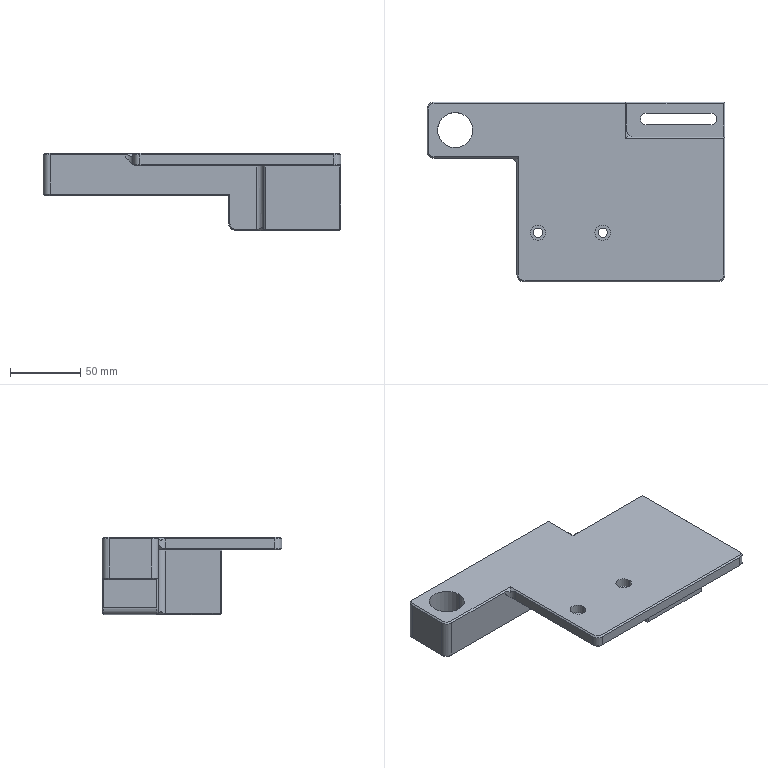NC program | NX | posted with a generic post | part box 212 x 128 x 55 mm
Lines 1 to 39 of 7327:
N10 G17 G21 G94 G90
(DRILLING_COPY_2 , TOOL : D8A45)
N12 T06 M6
N14 G54
N16 G17 G0 G90 X-86. Y44. S3000 M3
N18 G43 Z30. H6
N20 G94 G81 G98 Z-1. F150. R3.
N22 X-27. Y-29.
N24 X19.
N26 G80
N28 G0 X19. Y-29. Z30.
N30 M5
(DRILLING_COPY_COPY_COPY_COPY_1_COPY , TOOL : 6.6ZT)
N32 T15 M6
N34 G54
N36 G17 G0 G90 X-27. Y-29. S2000 M3
N38 G43 Z30. H15
N40 G94 G83 G98 Z-12.483 F100. Q2. R3.
N42 X19.
N44 G80
N46 G0 X19. Y-29. Z30.
N48 M5
(DRILLING_COPY_COPY_COPY_COPY_1_COPY_COPY , TOOL : 10.5ZT)
N50 T17 M6
N52 G54
N54 G17 G0 G90 X-86. Y44. S1000 M3
N56 G43 Z30. H17
N58 G94 G83 G98 Z-34.655 F100. Q2. R3.
N60 G80
N62 G0 X-86. Y44. Z30.
N64 M5